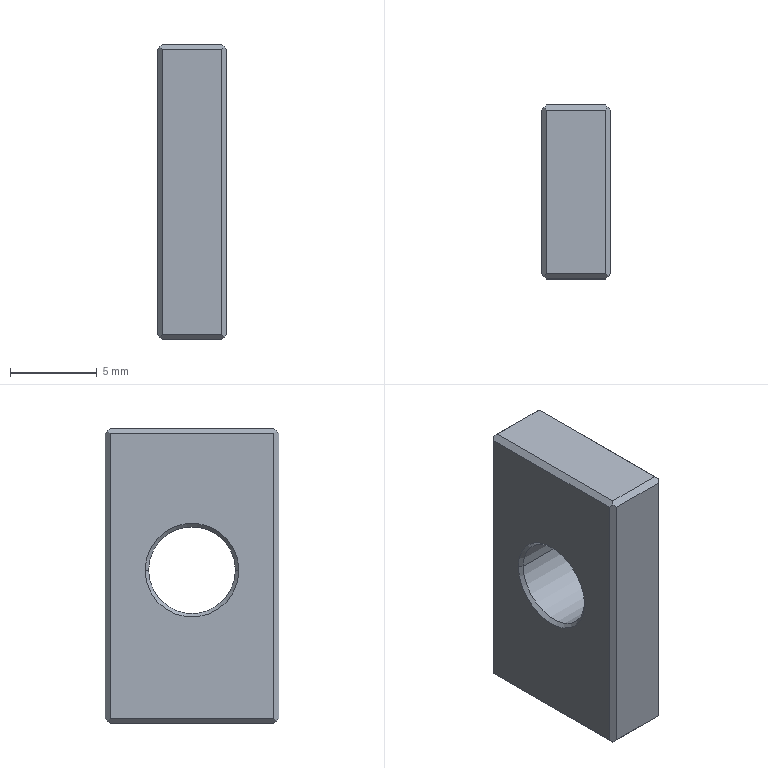Part | NX | 1 solid | 22 faces | box 4 x 10 x 17 mm | volume 595.72 mm3 | plane 18 | cylinder 2 | cone 2 | commonest cylinder face diameters 5 x2
STEP:
#1=CARTESIAN_POINT('',(2158.8,156.048,-140.3));
#2=VERTEX_POINT('',#1);
#3=CARTESIAN_POINT('',(2158.8,156.048,-156.7));
#4=VERTEX_POINT('',#3);
#5=CARTESIAN_POINT('',(2158.8,156.048,-148.5));
#6=DIRECTION('',(0.,0.,-1.));
#7=VECTOR('',#6,1000.);
#8=LINE('',#5,#7);
#9=EDGE_CURVE('',#2,#4,#8,.T.);
#10=ORIENTED_EDGE('',*,*,#9,.F.);
#11=CARTESIAN_POINT('',(2158.8,165.448,-140.3));
#12=VERTEX_POINT('',#11);
#13=CARTESIAN_POINT('',(2158.8,160.748,-140.3));
#14=DIRECTION('',(0.,1.,0.));
#15=VECTOR('',#14,1000.);
#16=LINE('',#13,#15);
#17=EDGE_CURVE('',#2,#12,#16,.T.);
#18=ORIENTED_EDGE('',*,*,#17,.T.);
#19=CARTESIAN_POINT('',(2158.8,165.448,-156.7));
#20=VERTEX_POINT('',#19);
#21=CARTESIAN_POINT('',(2158.8,165.448,-148.5));
#22=DIRECTION('',(0.,0.,1.));
#23=VECTOR('',#22,1000.);
#24=LINE('',#21,#23);
#25=EDGE_CURVE('',#20,#12,#24,.T.);
#26=ORIENTED_EDGE('',*,*,#25,.F.);
#27=CARTESIAN_POINT('',(2158.8,160.748,-156.7));
#28=DIRECTION('',(0.,1.,0.));
#29=VECTOR('',#28,1000.);
#30=LINE('',#27,#29);
#31=EDGE_CURVE('',#4,#20,#30,.T.);
#32=ORIENTED_EDGE('',*,*,#31,.F.);
#33=EDGE_LOOP('',(#10,#18,#26,#32));
#34=FACE_BOUND('',#33,.T.);
#35=CARTESIAN_POINT('',(2158.8,163.448,-148.165));
#36=VERTEX_POINT('',#35);
#37=CARTESIAN_POINT('',(2158.8,158.048,-148.165));
#38=VERTEX_POINT('',#37);
#39=CARTESIAN_POINT('',(2158.8,160.748,-148.165));
#40=DIRECTION('',(-1.,0.,0.));
#41=DIRECTION('',(0.,-1.,0.));
#42=AXIS2_PLACEMENT_3D('',#39,#40,#41);
#43=CIRCLE('',#42,2.7);
#44=EDGE_CURVE('',#36,#38,#43,.T.);
#45=ORIENTED_EDGE('',*,*,#44,.F.);
#46=CARTESIAN_POINT('',(2158.8,160.748,-148.165));
#47=DIRECTION('',(-1.,0.,0.));
#48=DIRECTION('',(0.,-1.,0.));
#49=AXIS2_PLACEMENT_3D('',#46,#47,#48);
#50=CIRCLE('',#49,2.7);
#51=EDGE_CURVE('',#38,#36,#50,.T.);
#52=ORIENTED_EDGE('',*,*,#51,.F.);
#53=EDGE_LOOP('',(#45,#52));
#54=FACE_BOUND('',#53,.T.);
#55=CARTESIAN_POINT('',(2158.8,165.748,-140.));
#56=DIRECTION('',(-1.,0.,0.));
#57=DIRECTION('',(0.,0.,1.));
#58=AXIS2_PLACEMENT_3D('',#55,#56,#57);
#59=PLANE('',#58);
#60=ADVANCED_FACE('',(#34,#54),#59,.T.);
#61=CARTESIAN_POINT('',(2162.5,165.748,-140.3));
#62=VERTEX_POINT('',#61);
#63=CARTESIAN_POINT('',(2162.5,165.748,-156.7));
#64=VERTEX_POINT('',#63);
#65=CARTESIAN_POINT('',(2162.5,165.748,-148.5));
#66=DIRECTION('',(0.,0.,-1.));
#67=VECTOR('',#66,1000.);
#68=LINE('',#65,#67);
#69=EDGE_CURVE('',#62,#64,#68,.T.);
#70=ORIENTED_EDGE('',*,*,#69,.T.);
#71=CARTESIAN_POINT('',(2159.1,165.748,-156.7));
#72=VERTEX_POINT('',#71);
#73=CARTESIAN_POINT('',(2160.8,165.748,-156.7));
#74=DIRECTION('',(-1.,0.,0.));
#75=VECTOR('',#74,1000.);
#76=LINE('',#73,#75);
#77=EDGE_CURVE('',#64,#72,#76,.T.);
#78=ORIENTED_EDGE('',*,*,#77,.T.);
#79=CARTESIAN_POINT('',(2159.1,165.748,-140.3));
#80=VERTEX_POINT('',#79);
#81=CARTESIAN_POINT('',(2159.1,165.748,-148.5));
#82=DIRECTION('',(0.,0.,1.));
#83=VECTOR('',#82,1000.);
#84=LINE('',#81,#83);
#85=EDGE_CURVE('',#72,#80,#84,.T.);
#86=ORIENTED_EDGE('',*,*,#85,.T.);
#87=CARTESIAN_POINT('',(2160.8,165.748,-140.3));
#88=DIRECTION('',(-1.,0.,0.));
#89=VECTOR('',#88,1000.);
#90=LINE('',#87,#89);
#91=EDGE_CURVE('',#62,#80,#90,.T.);
#92=ORIENTED_EDGE('',*,*,#91,.F.);
#93=EDGE_LOOP('',(#70,#78,#86,#92));
#94=FACE_BOUND('',#93,.T.);
#95=CARTESIAN_POINT('',(2162.8,165.748,-140.));
#96=DIRECTION('',(0.,1.,0.));
#97=DIRECTION('',(1.,0.,0.));
#98=AXIS2_PLACEMENT_3D('',#95,#96,#97);
#99=PLANE('',#98);
#100=ADVANCED_FACE('',(#94),#99,.T.);
#101=CARTESIAN_POINT('',(2162.8,156.048,-140.3));
#102=VERTEX_POINT('',#101);
#103=CARTESIAN_POINT('',(2162.8,156.048,-156.7));
#104=VERTEX_POINT('',#103);
#105=CARTESIAN_POINT('',(2162.8,156.048,-148.5));
#106=DIRECTION('',(0.,0.,-1.));
#107=VECTOR('',#106,1000.);
#108=LINE('',#105,#107);
#109=EDGE_CURVE('',#102,#104,#108,.T.);
#110=ORIENTED_EDGE('',*,*,#109,.T.);
#111=CARTESIAN_POINT('',(2162.8,165.448,-156.7));
#112=VERTEX_POINT('',#111);
#113=CARTESIAN_POINT('',(2162.8,160.748,-156.7));
#114=DIRECTION('',(0.,1.,0.));
#115=VECTOR('',#114,1000.);
#116=LINE('',#113,#115);
#117=EDGE_CURVE('',#104,#112,#116,.T.);
#118=ORIENTED_EDGE('',*,*,#117,.T.);
#119=CARTESIAN_POINT('',(2162.8,165.448,-140.3));
#120=VERTEX_POINT('',#119);
#121=CARTESIAN_POINT('',(2162.8,165.448,-148.5));
#122=DIRECTION('',(0.,0.,-1.));
#123=VECTOR('',#122,1000.);
#124=LINE('',#121,#123);
#125=EDGE_CURVE('',#120,#112,#124,.T.);
#126=ORIENTED_EDGE('',*,*,#125,.F.);
#127=CARTESIAN_POINT('',(2162.8,160.748,-140.3));
#128=DIRECTION('',(0.,1.,0.));
#129=VECTOR('',#128,1000.);
#130=LINE('',#127,#129);
#131=EDGE_CURVE('',#102,#120,#130,.T.);
#132=ORIENTED_EDGE('',*,*,#131,.F.);
#133=EDGE_LOOP('',(#110,#118,#126,#132));
#134=FACE_BOUND('',#133,.T.);
#135=CARTESIAN_POINT('',(2162.8,163.248,-148.165));
#136=VERTEX_POINT('',#135);
#137=CARTESIAN_POINT('',(2162.8,158.248,-148.165));
#138=VERTEX_POINT('',#137);
#139=CARTESIAN_POINT('',(2162.8,160.748,-148.165));
#140=DIRECTION('',(-1.,0.,0.));
#141=DIRECTION('',(0.,-1.,0.));
#142=AXIS2_PLACEMENT_3D('',#139,#140,#141);
#143=CIRCLE('',#142,2.5);
#144=EDGE_CURVE('',#136,#138,#143,.T.);
#145=ORIENTED_EDGE('',*,*,#144,.T.);
#146=CARTESIAN_POINT('',(2162.8,160.748,-148.165));
#147=DIRECTION('',(-1.,0.,0.));
#148=DIRECTION('',(0.,-1.,0.));
#149=AXIS2_PLACEMENT_3D('',#146,#147,#148);
#150=CIRCLE('',#149,2.5);
#151=EDGE_CURVE('',#138,#136,#150,.T.);
#152=ORIENTED_EDGE('',*,*,#151,.T.);
#153=EDGE_LOOP('',(#145,#152));
#154=FACE_BOUND('',#153,.T.);
#155=CARTESIAN_POINT('',(2162.8,155.748,-140.));
#156=DIRECTION('',(1.,0.,0.));
#157=DIRECTION('',(0.,1.,0.));
#158=AXIS2_PLACEMENT_3D('',#155,#156,#157);
#159=PLANE('',#158);
#160=ADVANCED_FACE('',(#134,#154),#159,.T.);
#161=CARTESIAN_POINT('',(2159.1,155.748,-140.3));
#162=VERTEX_POINT('',#161);
#163=CARTESIAN_POINT('',(2162.5,155.748,-140.3));
#164=VERTEX_POINT('',#163);
#165=CARTESIAN_POINT('',(2160.8,155.748,-140.3));
#166=DIRECTION('',(1.,0.,0.));
#167=VECTOR('',#166,1000.);
#168=LINE('',#165,#167);
#169=EDGE_CURVE('',#162,#164,#168,.T.);
#170=ORIENTED_EDGE('',*,*,#169,.F.);
#171=CARTESIAN_POINT('',(2159.1,155.748,-156.7));
#172=VERTEX_POINT('',#171);
#173=CARTESIAN_POINT('',(2159.1,155.748,-148.5));
#174=DIRECTION('',(0.,0.,-1.));
#175=VECTOR('',#174,1000.);
#176=LINE('',#173,#175);
#177=EDGE_CURVE('',#162,#172,#176,.T.);
#178=ORIENTED_EDGE('',*,*,#177,.T.);
#179=CARTESIAN_POINT('',(2162.5,155.748,-156.7));
#180=VERTEX_POINT('',#179);
#181=CARTESIAN_POINT('',(2160.8,155.748,-156.7));
#182=DIRECTION('',(1.,0.,0.));
#183=VECTOR('',#182,1000.);
#184=LINE('',#181,#183);
#185=EDGE_CURVE('',#172,#180,#184,.T.);
#186=ORIENTED_EDGE('',*,*,#185,.T.);
#187=CARTESIAN_POINT('',(2162.5,155.748,-148.5));
#188=DIRECTION('',(0.,0.,-1.));
#189=VECTOR('',#188,1000.);
#190=LINE('',#187,#189);
#191=EDGE_CURVE('',#164,#180,#190,.T.);
#192=ORIENTED_EDGE('',*,*,#191,.F.);
#193=EDGE_LOOP('',(#170,#178,#186,#192));
#194=FACE_BOUND('',#193,.T.);
#195=CARTESIAN_POINT('',(2157.8,155.748,-140.));
#196=DIRECTION('',(0.,-1.,0.));
#197=DIRECTION('',(0.,0.,-1.));
#198=AXIS2_PLACEMENT_3D('',#195,#196,#197);
#199=PLANE('',#198);
#200=ADVANCED_FACE('',(#194),#199,.T.);
#201=CARTESIAN_POINT('',(2159.,158.248,-148.165));
#202=VERTEX_POINT('',#201);
#203=CARTESIAN_POINT('',(2159.,163.248,-148.165));
#204=VERTEX_POINT('',#203);
#205=CARTESIAN_POINT('',(2159.,160.748,-148.165));
#206=DIRECTION('',(-1.,0.,0.));
#207=DIRECTION('',(0.,-1.,0.));
#208=AXIS2_PLACEMENT_3D('',#205,#206,#207);
#209=CIRCLE('',#208,2.5);
#210=EDGE_CURVE('',#202,#204,#209,.T.);
#211=ORIENTED_EDGE('',*,*,#210,.T.);
#212=CARTESIAN_POINT('',(2157.8,163.248,-148.165));
#213=DIRECTION('',(-1.,0.,0.));
#214=VECTOR('',#213,1000.);
#215=LINE('',#212,#214);
#216=EDGE_CURVE('',#136,#204,#215,.T.);
#217=ORIENTED_EDGE('',*,*,#216,.F.);
#218=ORIENTED_EDGE('',*,*,#151,.F.);
#219=CARTESIAN_POINT('',(2157.8,158.248,-148.165));
#220=DIRECTION('',(-1.,0.,0.));
#221=VECTOR('',#220,1000.);
#222=LINE('',#219,#221);
#223=EDGE_CURVE('',#138,#202,#222,.T.);
#224=ORIENTED_EDGE('',*,*,#223,.T.);
#225=EDGE_LOOP('',(#211,#217,#218,#224));
#226=FACE_BOUND('',#225,.T.);
#227=CARTESIAN_POINT('',(2157.8,160.748,-148.165));
#228=DIRECTION('',(-1.,0.,0.));
#229=DIRECTION('',(0.,-1.,0.));
#230=AXIS2_PLACEMENT_3D('',#227,#228,#229);
#231=CYLINDRICAL_SURFACE('',#230,2.5);
#232=ADVANCED_FACE('',(#226),#231,.F.);
#233=ORIENTED_EDGE('',*,*,#210,.F.);
#234=CARTESIAN_POINT('',(2159.,158.248,-148.165));
#235=DIRECTION('',(-0.7071,-0.7071,0.));
#236=VECTOR('',#235,1000.);
#237=LINE('',#234,#236);
#238=EDGE_CURVE('',#38,#202,#237,.F.);
#239=ORIENTED_EDGE('',*,*,#238,.F.);
#240=ORIENTED_EDGE('',*,*,#51,.T.);
#241=CARTESIAN_POINT('',(2159.,163.248,-148.165));
#242=DIRECTION('',(-0.7071,0.7071,0.));
#243=VECTOR('',#242,1000.);
#244=LINE('',#241,#243);
#245=EDGE_CURVE('',#36,#204,#244,.F.);
#246=ORIENTED_EDGE('',*,*,#245,.T.);
#247=EDGE_LOOP('',(#233,#239,#240,#246));
#248=FACE_BOUND('',#247,.T.);
#249=CARTESIAN_POINT('',(2159.,160.748,-148.165));
#250=DIRECTION('',(-1.,0.,0.));
#251=DIRECTION('',(0.,1.,0.));
#252=AXIS2_PLACEMENT_3D('',#249,#250,#251);
#253=CONICAL_SURFACE('',#252,2.5,0.7854);
#254=ADVANCED_FACE('',(#248),#253,.F.);
#255=ORIENTED_EDGE('',*,*,#25,.T.);
#256=CARTESIAN_POINT('',(2158.95,165.598,-140.15));
#257=VERTEX_POINT('',#256);
#258=CARTESIAN_POINT('',(2160.265,166.913,-138.835));
#259=DIRECTION('',(0.5774,0.5774,0.5774));
#260=VECTOR('',#259,1000.);
#261=LINE('',#258,#260);
#262=EDGE_CURVE('',#12,#257,#261,.T.);
#263=ORIENTED_EDGE('',*,*,#262,.T.);
#264=CARTESIAN_POINT('',(2158.8,165.448,-140.));
#265=DIRECTION('',(-0.5774,-0.5774,0.5774));
#266=VECTOR('',#265,1000.);
#267=LINE('',#264,#266);
#268=EDGE_CURVE('',#80,#257,#267,.T.);
#269=ORIENTED_EDGE('',*,*,#268,.F.);
#270=ORIENTED_EDGE('',*,*,#85,.F.);
#271=CARTESIAN_POINT('',(2158.95,165.598,-156.85));
#272=VERTEX_POINT('',#271);
#273=CARTESIAN_POINT('',(2175.8,182.448,-140.));
#274=DIRECTION('',(-0.5774,-0.5774,-0.5774));
#275=VECTOR('',#274,1000.);
#276=LINE('',#273,#275);
#277=EDGE_CURVE('',#72,#272,#276,.T.);
#278=ORIENTED_EDGE('',*,*,#277,.T.);
#279=CARTESIAN_POINT('',(2142.1,148.748,-140.));
#280=DIRECTION('',(-0.5774,-0.5774,0.5774));
#281=VECTOR('',#280,1000.);
#282=LINE('',#279,#281);
#283=EDGE_CURVE('',#272,#20,#282,.T.);
#284=ORIENTED_EDGE('',*,*,#283,.T.);
#285=EDGE_LOOP('',(#255,#263,#269,#270,#278,#284));
#286=FACE_BOUND('',#285,.T.);
#287=CARTESIAN_POINT('',(2158.95,165.598,-148.5));
#288=DIRECTION('',(0.7071,-0.7071,0.));
#289=DIRECTION('',(0.,0.,-1.));
#290=AXIS2_PLACEMENT_3D('',#287,#288,#289);
#291=PLANE('',#290);
#292=ADVANCED_FACE('',(#286),#291,.F.);
#293=ORIENTED_EDGE('',*,*,#69,.F.);
#294=CARTESIAN_POINT('',(2162.65,165.598,-140.15));
#295=VERTEX_POINT('',#294);
#296=CARTESIAN_POINT('',(2162.8,165.448,-140.));
#297=DIRECTION('',(-0.5774,0.5774,-0.5774));
#298=VECTOR('',#297,1000.);
#299=LINE('',#296,#298);
#300=EDGE_CURVE('',#295,#62,#299,.T.);
#301=ORIENTED_EDGE('',*,*,#300,.F.);
#302=CARTESIAN_POINT('',(2167.126,161.122,-144.626));
#303=DIRECTION('',(-0.5774,0.5774,0.5774));
#304=VECTOR('',#303,1000.);
#305=LINE('',#302,#304);
#306=EDGE_CURVE('',#120,#295,#305,.T.);
#307=ORIENTED_EDGE('',*,*,#306,.F.);
#308=ORIENTED_EDGE('',*,*,#125,.T.);
#309=CARTESIAN_POINT('',(2162.65,165.598,-156.85));
#310=VERTEX_POINT('',#309);
#311=CARTESIAN_POINT('',(2179.5,148.748,-140.));
#312=DIRECTION('',(0.5774,-0.5774,0.5774));
#313=VECTOR('',#312,1000.);
#314=LINE('',#311,#313);
#315=EDGE_CURVE('',#310,#112,#314,.T.);
#316=ORIENTED_EDGE('',*,*,#315,.F.);
#317=CARTESIAN_POINT('',(2145.8,182.448,-140.));
#318=DIRECTION('',(0.5774,-0.5774,-0.5774));
#319=VECTOR('',#318,1000.);
#320=LINE('',#317,#319);
#321=EDGE_CURVE('',#64,#310,#320,.T.);
#322=ORIENTED_EDGE('',*,*,#321,.F.);
#323=EDGE_LOOP('',(#293,#301,#307,#308,#316,#322));
#324=FACE_BOUND('',#323,.T.);
#325=CARTESIAN_POINT('',(2162.65,165.598,-148.5));
#326=DIRECTION('',(0.7071,0.7071,0.));
#327=DIRECTION('',(0.,0.,-1.));
#328=AXIS2_PLACEMENT_3D('',#325,#326,#327);
#329=PLANE('',#328);
#330=ADVANCED_FACE('',(#324),#329,.T.);
#331=ORIENTED_EDGE('',*,*,#109,.F.);
#332=CARTESIAN_POINT('',(2162.65,155.898,-140.15));
#333=VERTEX_POINT('',#332);
#334=CARTESIAN_POINT('',(2162.5,155.748,-140.));
#335=DIRECTION('',(0.5774,0.5774,-0.5774));
#336=VECTOR('',#335,1000.);
#337=LINE('',#334,#336);
#338=EDGE_CURVE('',#333,#102,#337,.T.);
#339=ORIENTED_EDGE('',*,*,#338,.F.);
#340=CARTESIAN_POINT('',(2162.8,156.048,-140.));
#341=DIRECTION('',(-0.5774,-0.5774,-0.5774));
#342=VECTOR('',#341,1000.);
#343=LINE('',#340,#342);
#344=EDGE_CURVE('',#333,#164,#343,.T.);
#345=ORIENTED_EDGE('',*,*,#344,.T.);
#346=ORIENTED_EDGE('',*,*,#191,.T.);
#347=CARTESIAN_POINT('',(2162.65,155.898,-156.85));
#348=VERTEX_POINT('',#347);
#349=CARTESIAN_POINT('',(2145.8,139.048,-140.));
#350=DIRECTION('',(0.5774,0.5774,-0.5774));
#351=VECTOR('',#350,1000.);
#352=LINE('',#349,#351);
#353=EDGE_CURVE('',#180,#348,#352,.T.);
#354=ORIENTED_EDGE('',*,*,#353,.T.);
#355=CARTESIAN_POINT('',(2179.5,172.748,-140.));
#356=DIRECTION('',(0.5774,0.5774,0.5774));
#357=VECTOR('',#356,1000.);
#358=LINE('',#355,#357);
#359=EDGE_CURVE('',#348,#104,#358,.T.);
#360=ORIENTED_EDGE('',*,*,#359,.T.);
#361=EDGE_LOOP('',(#331,#339,#345,#346,#354,#360));
#362=FACE_BOUND('',#361,.T.);
#363=CARTESIAN_POINT('',(2162.65,155.898,-148.5));
#364=DIRECTION('',(0.7071,-0.7071,0.));
#365=DIRECTION('',(0.,0.,-1.));
#366=AXIS2_PLACEMENT_3D('',#363,#364,#365);
#367=PLANE('',#366);
#368=ADVANCED_FACE('',(#362),#367,.T.);
#369=ORIENTED_EDGE('',*,*,#9,.T.);
#370=CARTESIAN_POINT('',(2158.95,155.898,-156.85));
#371=VERTEX_POINT('',#370);
#372=CARTESIAN_POINT('',(2142.1,172.748,-140.));
#373=DIRECTION('',(0.5774,-0.5774,-0.5774));
#374=VECTOR('',#373,1000.);
#375=LINE('',#372,#374);
#376=EDGE_CURVE('',#4,#371,#375,.T.);
#377=ORIENTED_EDGE('',*,*,#376,.T.);
#378=CARTESIAN_POINT('',(2175.8,139.048,-140.));
#379=DIRECTION('',(-0.5774,0.5774,-0.5774));
#380=VECTOR('',#379,1000.);
#381=LINE('',#378,#380);
#382=EDGE_CURVE('',#172,#371,#381,.T.);
#383=ORIENTED_EDGE('',*,*,#382,.F.);
#384=ORIENTED_EDGE('',*,*,#177,.F.);
#385=CARTESIAN_POINT('',(2158.95,155.898,-140.15));
#386=VERTEX_POINT('',#385);
#387=CARTESIAN_POINT('',(2158.8,156.048,-140.));
#388=DIRECTION('',(0.5774,-0.5774,-0.5774));
#389=VECTOR('',#388,1000.);
#390=LINE('',#387,#389);
#391=EDGE_CURVE('',#386,#162,#390,.T.);
#392=ORIENTED_EDGE('',*,*,#391,.F.);
#393=CARTESIAN_POINT('',(2153.726,161.122,-145.374));
#394=DIRECTION('',(0.5774,-0.5774,0.5774));
#395=VECTOR('',#394,1000.);
#396=LINE('',#393,#395);
#397=EDGE_CURVE('',#2,#386,#396,.T.);
#398=ORIENTED_EDGE('',*,*,#397,.F.);
#399=EDGE_LOOP('',(#369,#377,#383,#384,#392,#398));
#400=FACE_BOUND('',#399,.T.);
#401=CARTESIAN_POINT('',(2158.95,155.898,-148.5));
#402=DIRECTION('',(0.7071,0.7071,0.));
#403=DIRECTION('',(0.,0.,-1.));
#404=AXIS2_PLACEMENT_3D('',#401,#402,#403);
#405=PLANE('',#404);
#406=ADVANCED_FACE('',(#400),#405,.F.);
#407=CARTESIAN_POINT('',(2159.1,156.048,-140.));
#408=VERTEX_POINT('',#407);
#409=CARTESIAN_POINT('',(2162.5,156.048,-140.));
#410=VERTEX_POINT('',#409);
#411=CARTESIAN_POINT('',(2160.8,156.048,-140.));
#412=DIRECTION('',(1.,0.,0.));
#413=VECTOR('',#412,1000.);
#414=LINE('',#411,#413);
#415=EDGE_CURVE('',#408,#410,#414,.T.);
#416=ORIENTED_EDGE('',*,*,#415,.F.);
#417=CARTESIAN_POINT('',(2160.265,157.213,-138.835));
#418=DIRECTION('',(-0.5774,-0.5774,-0.5774));
#419=VECTOR('',#418,1000.);
#420=LINE('',#417,#419);
#421=EDGE_CURVE('',#408,#386,#420,.T.);
#422=ORIENTED_EDGE('',*,*,#421,.T.);
#423=ORIENTED_EDGE('',*,*,#391,.T.);
#424=ORIENTED_EDGE('',*,*,#169,.T.);
#425=ORIENTED_EDGE('',*,*,#344,.F.);
#426=CARTESIAN_POINT('',(2162.5,156.048,-140.));
#427=DIRECTION('',(0.5774,-0.5774,-0.5774));
#428=VECTOR('',#427,1000.);
#429=LINE('',#426,#428);
#430=EDGE_CURVE('',#410,#333,#429,.T.);
#431=ORIENTED_EDGE('',*,*,#430,.F.);
#432=EDGE_LOOP('',(#416,#422,#423,#424,#425,#431));
#433=FACE_BOUND('',#432,.T.);
#434=CARTESIAN_POINT('',(2160.8,155.898,-140.15));
#435=DIRECTION('',(0.,-0.7071,0.7071));
#436=DIRECTION('',(-1.,0.,0.));
#437=AXIS2_PLACEMENT_3D('',#434,#435,#436);
#438=PLANE('',#437);
#439=ADVANCED_FACE('',(#433),#438,.T.);
#440=CARTESIAN_POINT('',(2162.5,165.448,-140.));
#441=VERTEX_POINT('',#440);
#442=CARTESIAN_POINT('',(2159.1,165.448,-140.));
#443=VERTEX_POINT('',#442);
#444=CARTESIAN_POINT('',(2160.8,165.448,-140.));
#445=DIRECTION('',(-1.,0.,0.));
#446=VECTOR('',#445,1000.);
#447=LINE('',#444,#446);
#448=EDGE_CURVE('',#441,#443,#447,.T.);
#449=ORIENTED_EDGE('',*,*,#448,.F.);
#450=CARTESIAN_POINT('',(2162.5,165.448,-140.));
#451=DIRECTION('',(-0.5774,-0.5774,0.5774));
#452=VECTOR('',#451,1000.);
#453=LINE('',#450,#452);
#454=EDGE_CURVE('',#295,#441,#453,.T.);
#455=ORIENTED_EDGE('',*,*,#454,.F.);
#456=ORIENTED_EDGE('',*,*,#300,.T.);
#457=ORIENTED_EDGE('',*,*,#91,.T.);
#458=ORIENTED_EDGE('',*,*,#268,.T.);
#459=CARTESIAN_POINT('',(2160.265,164.282,-138.835));
#460=DIRECTION('',(0.5774,-0.5774,0.5774));
#461=VECTOR('',#460,1000.);
#462=LINE('',#459,#461);
#463=EDGE_CURVE('',#257,#443,#462,.T.);
#464=ORIENTED_EDGE('',*,*,#463,.T.);
#465=EDGE_LOOP('',(#449,#455,#456,#457,#458,#464));
#466=FACE_BOUND('',#465,.T.);
#467=CARTESIAN_POINT('',(2160.8,165.598,-140.15));
#468=DIRECTION('',(0.,0.7071,0.7071));
#469=DIRECTION('',(1.,0.,0.));
#470=AXIS2_PLACEMENT_3D('',#467,#468,#469);
#471=PLANE('',#470);
#472=ADVANCED_FACE('',(#466),#471,.T.);
#473=CARTESIAN_POINT('',(2159.1,156.048,-157.));
#474=VERTEX_POINT('',#473);
#475=CARTESIAN_POINT('',(2162.5,156.048,-157.));
#476=VERTEX_POINT('',#475);
#477=CARTESIAN_POINT('',(2160.8,156.048,-157.));
#478=DIRECTION('',(1.,0.,0.));
#479=VECTOR('',#478,1000.);
#480=LINE('',#477,#479);
#481=EDGE_CURVE('',#474,#476,#480,.T.);
#482=ORIENTED_EDGE('',*,*,#481,.F.);
#483=CARTESIAN_POINT('',(2159.1,165.448,-157.));
#484=VERTEX_POINT('',#483);
#485=CARTESIAN_POINT('',(2159.1,160.748,-157.));
#486=DIRECTION('',(0.,1.,0.));
#487=VECTOR('',#486,1000.);
#488=LINE('',#485,#487);
#489=EDGE_CURVE('',#474,#484,#488,.T.);
#490=ORIENTED_EDGE('',*,*,#489,.T.);
#491=CARTESIAN_POINT('',(2162.5,165.448,-157.));
#492=VERTEX_POINT('',#491);
#493=CARTESIAN_POINT('',(2160.8,165.448,-157.));
#494=DIRECTION('',(-1.,0.,0.));
#495=VECTOR('',#494,1000.);
#496=LINE('',#493,#495);
#497=EDGE_CURVE('',#492,#484,#496,.T.);
#498=ORIENTED_EDGE('',*,*,#497,.F.);
#499=CARTESIAN_POINT('',(2162.5,160.748,-157.));
#500=DIRECTION('',(0.,1.,0.));
#501=VECTOR('',#500,1000.);
#502=LINE('',#499,#501);
#503=EDGE_CURVE('',#476,#492,#502,.T.);
#504=ORIENTED_EDGE('',*,*,#503,.F.);
#505=EDGE_LOOP('',(#482,#490,#498,#504));
#506=FACE_BOUND('',#505,.T.);
#507=CARTESIAN_POINT('',(2160.265,161.122,-157.));
#508=DIRECTION('',(0.,0.,-1.));
#509=DIRECTION('',(0.,-1.,0.));
#510=AXIS2_PLACEMENT_3D('',#507,#508,#509);
#511=PLANE('',#510);
#512=ADVANCED_FACE('',(#506),#511,.T.);
#513=ORIENTED_EDGE('',*,*,#489,.F.);
#514=CARTESIAN_POINT('',(2142.1,139.048,-140.));
#515=DIRECTION('',(0.5774,0.5774,-0.5774));
#516=VECTOR('',#515,1000.);
#517=LINE('',#514,#516);
#518=EDGE_CURVE('',#371,#474,#517,.T.);
#519=ORIENTED_EDGE('',*,*,#518,.F.);
#520=ORIENTED_EDGE('',*,*,#376,.F.);
#521=ORIENTED_EDGE('',*,*,#31,.T.);
#522=ORIENTED_EDGE('',*,*,#283,.F.);
#523=CARTESIAN_POINT('',(2142.1,182.448,-140.));
#524=DIRECTION('',(-0.5774,0.5774,0.5774));
#525=VECTOR('',#524,1000.);
#526=LINE('',#523,#525);
#527=EDGE_CURVE('',#484,#272,#526,.T.);
#528=ORIENTED_EDGE('',*,*,#527,.F.);
#529=EDGE_LOOP('',(#513,#519,#520,#521,#522,#528));
#530=FACE_BOUND('',#529,.T.);
#531=CARTESIAN_POINT('',(2158.95,160.748,-156.85));
#532=DIRECTION('',(-0.7071,0.,-0.7071));
#533=DIRECTION('',(-0.7071,0.,0.7071));
#534=AXIS2_PLACEMENT_3D('',#531,#532,#533);
#535=PLANE('',#534);
#536=ADVANCED_FACE('',(#530),#535,.T.);
#537=ORIENTED_EDGE('',*,*,#497,.T.);
#538=ORIENTED_EDGE('',*,*,#527,.T.);
#539=ORIENTED_EDGE('',*,*,#277,.F.);
#540=ORIENTED_EDGE('',*,*,#77,.F.);
#541=ORIENTED_EDGE('',*,*,#321,.T.);
#542=CARTESIAN_POINT('',(2179.5,182.448,-140.));
#543=DIRECTION('',(-0.5774,-0.5774,-0.5774));
#544=VECTOR('',#543,1000.);
#545=LINE('',#542,#544);
#546=EDGE_CURVE('',#310,#492,#545,.T.);
#547=ORIENTED_EDGE('',*,*,#546,.T.);
#548=EDGE_LOOP('',(#537,#538,#539,#540,#541,#547));
#549=FACE_BOUND('',#548,.T.);
#550=CARTESIAN_POINT('',(2160.8,165.598,-156.85));
#551=DIRECTION('',(0.,-0.7071,0.7071));
#552=DIRECTION('',(-1.,0.,0.));
#553=AXIS2_PLACEMENT_3D('',#550,#551,#552);
#554=PLANE('',#553);
#555=ADVANCED_FACE('',(#549),#554,.F.);
#556=ORIENTED_EDGE('',*,*,#503,.T.);
#557=ORIENTED_EDGE('',*,*,#546,.F.);
#558=ORIENTED_EDGE('',*,*,#315,.T.);
#559=ORIENTED_EDGE('',*,*,#117,.F.);
#560=ORIENTED_EDGE('',*,*,#359,.F.);
#561=CARTESIAN_POINT('',(2179.5,139.048,-140.));
#562=DIRECTION('',(-0.5774,0.5774,-0.5774));
#563=VECTOR('',#562,1000.);
#564=LINE('',#561,#563);
#565=EDGE_CURVE('',#348,#476,#564,.T.);
#566=ORIENTED_EDGE('',*,*,#565,.T.);
#567=EDGE_LOOP('',(#556,#557,#558,#559,#560,#566));
#568=FACE_BOUND('',#567,.T.);
#569=CARTESIAN_POINT('',(2162.65,160.748,-156.85));
#570=DIRECTION('',(-0.7071,0.,0.7071));
#571=DIRECTION('',(0.,1.,0.));
#572=AXIS2_PLACEMENT_3D('',#569,#570,#571);
#573=PLANE('',#572);
#574=ADVANCED_FACE('',(#568),#573,.F.);
#575=ORIENTED_EDGE('',*,*,#481,.T.);
#576=ORIENTED_EDGE('',*,*,#565,.F.);
#577=ORIENTED_EDGE('',*,*,#353,.F.);
#578=ORIENTED_EDGE('',*,*,#185,.F.);
#579=ORIENTED_EDGE('',*,*,#382,.T.);
#580=ORIENTED_EDGE('',*,*,#518,.T.);
#581=EDGE_LOOP('',(#575,#576,#577,#578,#579,#580));
#582=FACE_BOUND('',#581,.T.);
#583=CARTESIAN_POINT('',(2160.8,155.898,-156.85));
#584=DIRECTION('',(0.,0.7071,0.7071));
#585=DIRECTION('',(1.,0.,0.));
#586=AXIS2_PLACEMENT_3D('',#583,#584,#585);
#587=PLANE('',#586);
#588=ADVANCED_FACE('',(#582),#587,.F.);
#589=ORIENTED_EDGE('',*,*,#415,.T.);
#590=CARTESIAN_POINT('',(2162.5,160.748,-140.));
#591=DIRECTION('',(0.,1.,0.));
#592=VECTOR('',#591,1000.);
#593=LINE('',#590,#592);
#594=EDGE_CURVE('',#410,#441,#593,.T.);
#595=ORIENTED_EDGE('',*,*,#594,.T.);
#596=ORIENTED_EDGE('',*,*,#448,.T.);
#597=CARTESIAN_POINT('',(2159.1,160.748,-140.));
#598=DIRECTION('',(0.,1.,0.));
#599=VECTOR('',#598,1000.);
#600=LINE('',#597,#599);
#601=EDGE_CURVE('',#408,#443,#600,.T.);
#602=ORIENTED_EDGE('',*,*,#601,.F.);
#603=EDGE_LOOP('',(#589,#595,#596,#602));
#604=FACE_BOUND('',#603,.T.);
#605=CARTESIAN_POINT('',(2160.265,161.122,-140.));
#606=DIRECTION('',(0.,0.,-1.));
#607=DIRECTION('',(0.,-1.,0.));
#608=AXIS2_PLACEMENT_3D('',#605,#606,#607);
#609=PLANE('',#608);
#610=ADVANCED_FACE('',(#604),#609,.F.);
#611=ORIENTED_EDGE('',*,*,#601,.T.);
#612=ORIENTED_EDGE('',*,*,#463,.F.);
#613=ORIENTED_EDGE('',*,*,#262,.F.);
#614=ORIENTED_EDGE('',*,*,#17,.F.);
#615=ORIENTED_EDGE('',*,*,#397,.T.);
#616=ORIENTED_EDGE('',*,*,#421,.F.);
#617=EDGE_LOOP('',(#611,#612,#613,#614,#615,#616));
#618=FACE_BOUND('',#617,.T.);
#619=CARTESIAN_POINT('',(2158.95,160.748,-140.15));
#620=DIRECTION('',(0.7071,0.,-0.7071));
#621=DIRECTION('',(0.,-1.,0.));
#622=AXIS2_PLACEMENT_3D('',#619,#620,#621);
#623=PLANE('',#622);
#624=ADVANCED_FACE('',(#618),#623,.F.);
#625=ORIENTED_EDGE('',*,*,#594,.F.);
#626=ORIENTED_EDGE('',*,*,#430,.T.);
#627=ORIENTED_EDGE('',*,*,#338,.T.);
#628=ORIENTED_EDGE('',*,*,#131,.T.);
#629=ORIENTED_EDGE('',*,*,#306,.T.);
#630=ORIENTED_EDGE('',*,*,#454,.T.);
#631=EDGE_LOOP('',(#625,#626,#627,#628,#629,#630));
#632=FACE_BOUND('',#631,.T.);
#633=CARTESIAN_POINT('',(2162.65,160.748,-140.15));
#634=DIRECTION('',(0.7071,0.,0.7071));
#635=DIRECTION('',(0.,-1.,0.));
#636=AXIS2_PLACEMENT_3D('',#633,#634,#635);
#637=PLANE('',#636);
#638=ADVANCED_FACE('',(#632),#637,.T.);
#639=ORIENTED_EDGE('',*,*,#144,.F.);
#640=ORIENTED_EDGE('',*,*,#216,.T.);
#641=CARTESIAN_POINT('',(2159.,160.748,-148.165));
#642=DIRECTION('',(-1.,0.,0.));
#643=DIRECTION('',(0.,-1.,0.));
#644=AXIS2_PLACEMENT_3D('',#641,#642,#643);
#645=CIRCLE('',#644,2.5);
#646=EDGE_CURVE('',#204,#202,#645,.T.);
#647=ORIENTED_EDGE('',*,*,#646,.T.);
#648=ORIENTED_EDGE('',*,*,#223,.F.);
#649=EDGE_LOOP('',(#639,#640,#647,#648));
#650=FACE_BOUND('',#649,.T.);
#651=CARTESIAN_POINT('',(2157.8,160.748,-148.165));
#652=DIRECTION('',(-1.,0.,0.));
#653=DIRECTION('',(0.,-1.,0.));
#654=AXIS2_PLACEMENT_3D('',#651,#652,#653);
#655=CYLINDRICAL_SURFACE('',#654,2.5);
#656=ADVANCED_FACE('',(#650),#655,.F.);
#657=ORIENTED_EDGE('',*,*,#44,.T.);
#658=ORIENTED_EDGE('',*,*,#238,.T.);
#659=ORIENTED_EDGE('',*,*,#646,.F.);
#660=ORIENTED_EDGE('',*,*,#245,.F.);
#661=EDGE_LOOP('',(#657,#658,#659,#660));
#662=FACE_BOUND('',#661,.T.);
#663=CARTESIAN_POINT('',(2159.,160.748,-148.165));
#664=DIRECTION('',(-1.,0.,0.));
#665=DIRECTION('',(0.,1.,0.));
#666=AXIS2_PLACEMENT_3D('',#663,#664,#665);
#667=CONICAL_SURFACE('',#666,2.5,0.7854);
#668=ADVANCED_FACE('',(#662),#667,.F.);
#669=CLOSED_SHELL('',(#60,#100,#160,#200,#232,#254,#292,#330,#368,#406,#439,#472,#512,#536,#555,#574,#588,#610,#624,#638,#656,#668));
#670=MANIFOLD_SOLID_BREP('',#669);
#671=(LENGTH_UNIT()NAMED_UNIT(*)SI_UNIT(.MILLI.,.METRE.));
#672=UNCERTAINTY_MEASURE_WITH_UNIT(LENGTH_MEASURE(0.00001),#671,'','');
#673=(NAMED_UNIT(*)PLANE_ANGLE_UNIT()SI_UNIT($,.RADIAN.));
#674=(NAMED_UNIT(*)SI_UNIT($,.STERADIAN.)SOLID_ANGLE_UNIT());
#675=(GEOMETRIC_REPRESENTATION_CONTEXT(3)GLOBAL_UNCERTAINTY_ASSIGNED_CONTEXT((#672))GLOBAL_UNIT_ASSIGNED_CONTEXT((#671,#673,#674))REPRESENTATION_CONTEXT('',''));
#676=ADVANCED_BREP_SHAPE_REPRESENTATION('',(#670),#675);